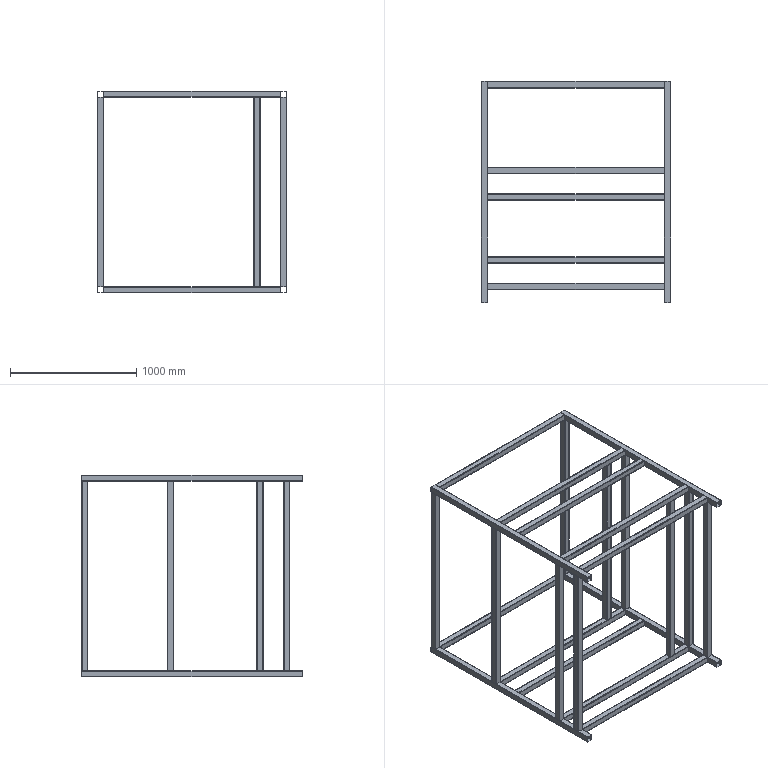Part | SolidWorks | features 3DProfileFeature 1, WeldCornerFeat 1, WeldMemberFeat 1, WeldmentFeature 1 | 24 solids | 432 faces | box 1500 x 1750 x 1600 mm | volume 13453168 mm3 | plane 240 | cylinder 192 | commonest cylinder face diameters 4 x96 8 x96